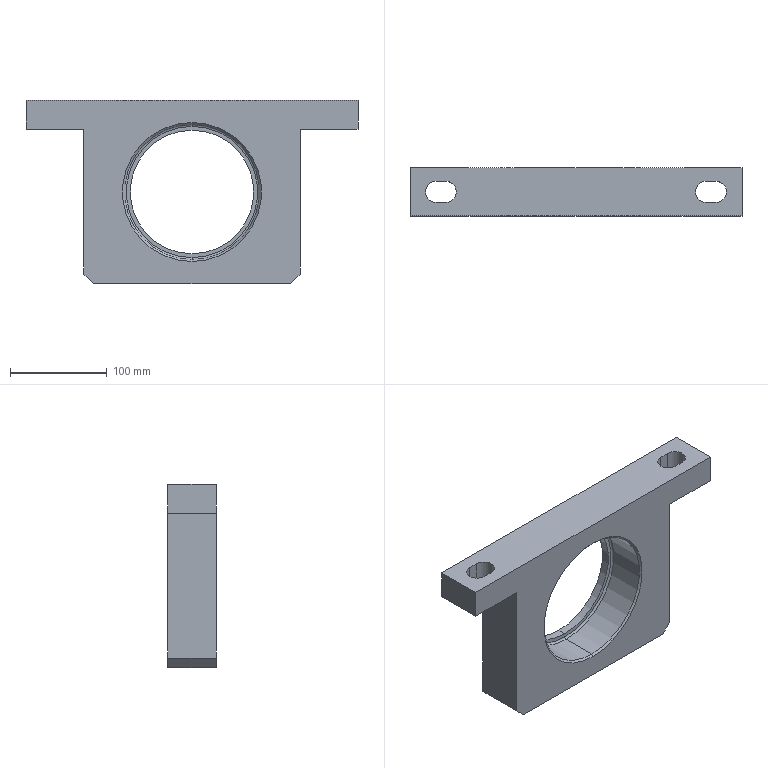Part | SolidWorks | features ICE 3, Chamfer 2, Extrusion 1, Fillet 1 | 1 solid | 31 faces | box 344 x 50 x 190 mm | volume 1518259 mm3 | plane 17 | cylinder 10 | torus 2 | cone 2 | commonest cylinder face diameters 22 x6 128 x2 140 x2
STEP:
#1=CARTESIAN_POINT('',(-156.,0.,0.));
#2=VERTEX_POINT('',#1);
#3=CARTESIAN_POINT('',(-145.,11.,0.));
#4=VERTEX_POINT('',#3);
#5=CARTESIAN_POINT('',(-145.,0.,0.));
#6=DIRECTION('',(0.,0.,-1.));
#7=DIRECTION('',(-1.,0.,0.));
#8=AXIS2_PLACEMENT_3D('',#5,#6,#7);
#9=CIRCLE('',#8,11.);
#10=EDGE_CURVE('',#2,#4,#9,.T.);
#11=ORIENTED_EDGE('',*,*,#10,.F.);
#12=CARTESIAN_POINT('',(-156.,0.,-30.));
#13=VERTEX_POINT('',#12);
#14=CARTESIAN_POINT('',(-156.,0.,11.5));
#15=DIRECTION('',(0.,0.,-1.));
#16=VECTOR('',#15,1000.);
#17=LINE('',#14,#16);
#18=EDGE_CURVE('',#2,#13,#17,.T.);
#19=ORIENTED_EDGE('',*,*,#18,.T.);
#20=CARTESIAN_POINT('',(-145.,11.,-30.));
#21=VERTEX_POINT('',#20);
#22=CARTESIAN_POINT('',(-145.,0.,-30.));
#23=DIRECTION('',(0.,0.,-1.));
#24=DIRECTION('',(-1.,0.,0.));
#25=AXIS2_PLACEMENT_3D('',#22,#23,#24);
#26=CIRCLE('',#25,11.);
#27=EDGE_CURVE('',#13,#21,#26,.T.);
#28=ORIENTED_EDGE('',*,*,#27,.T.);
#29=CARTESIAN_POINT('',(-145.,11.,11.5));
#30=DIRECTION('',(0.,0.,-1.));
#31=VECTOR('',#30,1000.);
#32=LINE('',#29,#31);
#33=EDGE_CURVE('',#4,#21,#32,.T.);
#34=ORIENTED_EDGE('',*,*,#33,.F.);
#35=EDGE_LOOP('',(#11,#19,#28,#34));
#36=FACE_OUTER_BOUND('',#35,.T.);
#37=CARTESIAN_POINT('',(-145.,0.,11.5));
#38=DIRECTION('',(0.,0.,-1.));
#39=DIRECTION('',(-1.,0.,0.));
#40=AXIS2_PLACEMENT_3D('',#37,#38,#39);
#41=CYLINDRICAL_SURFACE('',#40,11.);
#42=ADVANCED_FACE('',(#36),#41,.F.);
#43=CARTESIAN_POINT('',(124.,0.,0.));
#44=VERTEX_POINT('',#43);
#45=CARTESIAN_POINT('',(135.,11.,0.));
#46=VERTEX_POINT('',#45);
#47=CARTESIAN_POINT('',(135.,0.,0.));
#48=DIRECTION('',(0.,0.,-1.));
#49=DIRECTION('',(-1.,0.,0.));
#50=AXIS2_PLACEMENT_3D('',#47,#48,#49);
#51=CIRCLE('',#50,11.);
#52=EDGE_CURVE('',#44,#46,#51,.T.);
#53=ORIENTED_EDGE('',*,*,#52,.F.);
#54=CARTESIAN_POINT('',(124.,0.,-30.));
#55=VERTEX_POINT('',#54);
#56=CARTESIAN_POINT('',(124.,0.,11.5));
#57=DIRECTION('',(0.,0.,-1.));
#58=VECTOR('',#57,1000.);
#59=LINE('',#56,#58);
#60=EDGE_CURVE('',#44,#55,#59,.T.);
#61=ORIENTED_EDGE('',*,*,#60,.T.);
#62=CARTESIAN_POINT('',(135.,11.,-30.));
#63=VERTEX_POINT('',#62);
#64=CARTESIAN_POINT('',(135.,0.,-30.));
#65=DIRECTION('',(0.,0.,-1.));
#66=DIRECTION('',(-1.,0.,0.));
#67=AXIS2_PLACEMENT_3D('',#64,#65,#66);
#68=CIRCLE('',#67,11.);
#69=EDGE_CURVE('',#55,#63,#68,.T.);
#70=ORIENTED_EDGE('',*,*,#69,.T.);
#71=CARTESIAN_POINT('',(135.,11.,11.5));
#72=DIRECTION('',(0.,0.,-1.));
#73=VECTOR('',#72,1000.);
#74=LINE('',#71,#73);
#75=EDGE_CURVE('',#46,#63,#74,.T.);
#76=ORIENTED_EDGE('',*,*,#75,.F.);
#77=EDGE_LOOP('',(#53,#61,#70,#76));
#78=FACE_OUTER_BOUND('',#77,.T.);
#79=CARTESIAN_POINT('',(135.,0.,11.5));
#80=DIRECTION('',(0.,0.,-1.));
#81=DIRECTION('',(-1.,0.,0.));
#82=AXIS2_PLACEMENT_3D('',#79,#80,#81);
#83=CYLINDRICAL_SURFACE('',#82,11.);
#84=ADVANCED_FACE('',(#78),#83,.F.);
#85=CARTESIAN_POINT('',(0.,16.5,-27.));
#86=VERTEX_POINT('',#85);
#87=CARTESIAN_POINT('',(0.,16.5,-163.));
#88=VERTEX_POINT('',#87);
#89=CARTESIAN_POINT('',(0.,16.5,-95.));
#90=DIRECTION('',(0.,-1.,0.));
#91=DIRECTION('',(0.,0.,-1.));
#92=AXIS2_PLACEMENT_3D('',#89,#90,#91);
#93=CIRCLE('',#92,68.);
#94=EDGE_CURVE('',#86,#88,#93,.T.);
#95=ORIENTED_EDGE('',*,*,#94,.F.);
#96=CARTESIAN_POINT('',(0.,14.5,-25.));
#97=VERTEX_POINT('',#96);
#98=CARTESIAN_POINT('',(0.,14.5,-27.));
#99=DIRECTION('',(1.,0.,0.));
#100=DIRECTION('',(0.,0.,-1.));
#101=AXIS2_PLACEMENT_3D('',#98,#99,#100);
#102=CIRCLE('',#101,2.);
#103=EDGE_CURVE('',#86,#97,#102,.T.);
#104=ORIENTED_EDGE('',*,*,#103,.T.);
#105=CARTESIAN_POINT('',(0.,14.5,-165.));
#106=VERTEX_POINT('',#105);
#107=CARTESIAN_POINT('',(0.,14.5,-95.));
#108=DIRECTION('',(0.,1.,0.));
#109=DIRECTION('',(0.,0.,-1.));
#110=AXIS2_PLACEMENT_3D('',#107,#108,#109);
#111=CIRCLE('',#110,70.);
#112=EDGE_CURVE('',#106,#97,#111,.T.);
#113=ORIENTED_EDGE('',*,*,#112,.F.);
#114=CARTESIAN_POINT('',(0.,14.5,-163.));
#115=DIRECTION('',(-1.,0.,0.));
#116=DIRECTION('',(0.,0.,1.));
#117=AXIS2_PLACEMENT_3D('',#114,#115,#116);
#118=CIRCLE('',#117,2.);
#119=EDGE_CURVE('',#88,#106,#118,.T.);
#120=ORIENTED_EDGE('',*,*,#119,.F.);
#121=EDGE_LOOP('',(#95,#104,#113,#120));
#122=FACE_OUTER_BOUND('',#121,.T.);
#123=CARTESIAN_POINT('',(0.,14.5,-95.));
#124=DIRECTION('',(0.,-1.,0.));
#125=DIRECTION('',(0.,0.,-1.));
#126=AXIS2_PLACEMENT_3D('',#123,#124,#125);
#127=TOROIDAL_SURFACE('',#126,68.,2.);
#128=ADVANCED_FACE('',(#122),#127,.F.);
#129=CARTESIAN_POINT('',(0.,-23.,-25.));
#130=VERTEX_POINT('',#129);
#131=CARTESIAN_POINT('',(0.,-23.,-165.));
#132=VERTEX_POINT('',#131);
#133=CARTESIAN_POINT('',(0.,-23.,-95.));
#134=DIRECTION('',(0.,-1.,0.));
#135=DIRECTION('',(0.,0.,1.));
#136=AXIS2_PLACEMENT_3D('',#133,#134,#135);
#137=CIRCLE('',#136,70.);
#138=EDGE_CURVE('',#130,#132,#137,.T.);
#139=ORIENTED_EDGE('',*,*,#138,.F.);
#140=CARTESIAN_POINT('',(0.,-25.,-23.));
#141=VERTEX_POINT('',#140);
#142=CARTESIAN_POINT('',(0.,-23.,-25.));
#143=DIRECTION('',(0.,-0.7071,0.7071));
#144=VECTOR('',#143,1000.);
#145=LINE('',#142,#144);
#146=EDGE_CURVE('',#130,#141,#145,.T.);
#147=ORIENTED_EDGE('',*,*,#146,.T.);
#148=CARTESIAN_POINT('',(0.,-25.,-167.));
#149=VERTEX_POINT('',#148);
#150=CARTESIAN_POINT('',(0.,-25.,-95.));
#151=DIRECTION('',(0.,1.,0.));
#152=DIRECTION('',(0.,0.,1.));
#153=AXIS2_PLACEMENT_3D('',#150,#151,#152);
#154=CIRCLE('',#153,72.);
#155=EDGE_CURVE('',#149,#141,#154,.T.);
#156=ORIENTED_EDGE('',*,*,#155,.F.);
#157=CARTESIAN_POINT('',(0.,-23.,-165.));
#158=DIRECTION('',(0.,-0.7071,-0.7071));
#159=VECTOR('',#158,1000.);
#160=LINE('',#157,#159);
#161=EDGE_CURVE('',#132,#149,#160,.T.);
#162=ORIENTED_EDGE('',*,*,#161,.F.);
#163=EDGE_LOOP('',(#139,#147,#156,#162));
#164=FACE_OUTER_BOUND('',#163,.T.);
#165=CARTESIAN_POINT('',(0.,-23.,-95.));
#166=DIRECTION('',(0.,-1.,0.));
#167=DIRECTION('',(0.,0.,-1.));
#168=AXIS2_PLACEMENT_3D('',#165,#166,#167);
#169=CONICAL_SURFACE('',#168,70.,0.7854);
#170=ADVANCED_FACE('',(#164),#169,.F.);
#171=ORIENTED_EDGE('',*,*,#112,.T.);
#172=CARTESIAN_POINT('',(0.,16.5,-25.));
#173=DIRECTION('',(0.,-1.,0.));
#174=VECTOR('',#173,1000.);
#175=LINE('',#172,#174);
#176=EDGE_CURVE('',#97,#130,#175,.T.);
#177=ORIENTED_EDGE('',*,*,#176,.T.);
#178=ORIENTED_EDGE('',*,*,#138,.T.);
#179=CARTESIAN_POINT('',(0.,16.5,-165.));
#180=DIRECTION('',(0.,-1.,0.));
#181=VECTOR('',#180,1000.);
#182=LINE('',#179,#181);
#183=EDGE_CURVE('',#106,#132,#182,.T.);
#184=ORIENTED_EDGE('',*,*,#183,.F.);
#185=EDGE_LOOP('',(#171,#177,#178,#184));
#186=FACE_OUTER_BOUND('',#185,.T.);
#187=CARTESIAN_POINT('',(0.,16.5,-95.));
#188=DIRECTION('',(0.,-1.,0.));
#189=DIRECTION('',(0.,0.,-1.));
#190=AXIS2_PLACEMENT_3D('',#187,#188,#189);
#191=CYLINDRICAL_SURFACE('',#190,70.);
#192=ADVANCED_FACE('',(#186),#191,.F.);
#193=CARTESIAN_POINT('',(0.,25.,-159.));
#194=VERTEX_POINT('',#193);
#195=CARTESIAN_POINT('',(0.,25.,-31.));
#196=VERTEX_POINT('',#195);
#197=CARTESIAN_POINT('',(0.,25.,-95.));
#198=DIRECTION('',(0.,1.,0.));
#199=DIRECTION('',(0.,0.,1.));
#200=AXIS2_PLACEMENT_3D('',#197,#198,#199);
#201=CIRCLE('',#200,64.);
#202=EDGE_CURVE('',#194,#196,#201,.T.);
#203=ORIENTED_EDGE('',*,*,#202,.T.);
#204=CARTESIAN_POINT('',(0.,16.5,-31.));
#205=VERTEX_POINT('',#204);
#206=CARTESIAN_POINT('',(0.,25.,-31.));
#207=DIRECTION('',(0.,-1.,0.));
#208=VECTOR('',#207,1000.);
#209=LINE('',#206,#208);
#210=EDGE_CURVE('',#196,#205,#209,.T.);
#211=ORIENTED_EDGE('',*,*,#210,.T.);
#212=CARTESIAN_POINT('',(0.,16.5,-159.));
#213=VERTEX_POINT('',#212);
#214=CARTESIAN_POINT('',(0.,16.5,-95.));
#215=DIRECTION('',(0.,-1.,0.));
#216=DIRECTION('',(0.,0.,-1.));
#217=AXIS2_PLACEMENT_3D('',#214,#215,#216);
#218=CIRCLE('',#217,64.);
#219=EDGE_CURVE('',#205,#213,#218,.T.);
#220=ORIENTED_EDGE('',*,*,#219,.T.);
#221=CARTESIAN_POINT('',(0.,25.,-159.));
#222=DIRECTION('',(0.,-1.,0.));
#223=VECTOR('',#222,1000.);
#224=LINE('',#221,#223);
#225=EDGE_CURVE('',#194,#213,#224,.T.);
#226=ORIENTED_EDGE('',*,*,#225,.F.);
#227=EDGE_LOOP('',(#203,#211,#220,#226));
#228=FACE_OUTER_BOUND('',#227,.T.);
#229=CARTESIAN_POINT('',(0.,25.,-95.));
#230=DIRECTION('',(0.,-1.,0.));
#231=DIRECTION('',(0.,0.,-1.));
#232=AXIS2_PLACEMENT_3D('',#229,#230,#231);
#233=CYLINDRICAL_SURFACE('',#232,64.);
#234=ADVANCED_FACE('',(#228),#233,.F.);
#235=ORIENTED_EDGE('',*,*,#210,.F.);
#236=CARTESIAN_POINT('',(0.,25.,-95.));
#237=DIRECTION('',(0.,1.,0.));
#238=DIRECTION('',(0.,0.,1.));
#239=AXIS2_PLACEMENT_3D('',#236,#237,#238);
#240=CIRCLE('',#239,64.);
#241=EDGE_CURVE('',#196,#194,#240,.T.);
#242=ORIENTED_EDGE('',*,*,#241,.T.);
#243=ORIENTED_EDGE('',*,*,#225,.T.);
#244=CARTESIAN_POINT('',(0.,16.5,-95.));
#245=DIRECTION('',(0.,-1.,0.));
#246=DIRECTION('',(0.,0.,-1.));
#247=AXIS2_PLACEMENT_3D('',#244,#245,#246);
#248=CIRCLE('',#247,64.);
#249=EDGE_CURVE('',#213,#205,#248,.T.);
#250=ORIENTED_EDGE('',*,*,#249,.T.);
#251=EDGE_LOOP('',(#235,#242,#243,#250));
#252=FACE_OUTER_BOUND('',#251,.T.);
#253=CARTESIAN_POINT('',(0.,25.,-95.));
#254=DIRECTION('',(0.,-1.,0.));
#255=DIRECTION('',(0.,0.,-1.));
#256=AXIS2_PLACEMENT_3D('',#253,#254,#255);
#257=CYLINDRICAL_SURFACE('',#256,64.);
#258=ADVANCED_FACE('',(#252),#257,.F.);
#259=CARTESIAN_POINT('',(-102.,25.,-190.));
#260=VERTEX_POINT('',#259);
#261=CARTESIAN_POINT('',(102.,25.,-190.));
#262=VERTEX_POINT('',#261);
#263=CARTESIAN_POINT('',(-112.,25.,-190.));
#264=DIRECTION('',(1.,0.,0.));
#265=VECTOR('',#264,1000.);
#266=LINE('',#263,#265);
#267=EDGE_CURVE('',#260,#262,#266,.T.);
#268=ORIENTED_EDGE('',*,*,#267,.F.);
#269=CARTESIAN_POINT('',(-112.,25.,-180.));
#270=VERTEX_POINT('',#269);
#271=CARTESIAN_POINT('',(-98.5,25.,-193.5));
#272=DIRECTION('',(-0.7071,0.,0.7071));
#273=VECTOR('',#272,1000.);
#274=LINE('',#271,#273);
#275=EDGE_CURVE('',#260,#270,#274,.T.);
#276=ORIENTED_EDGE('',*,*,#275,.T.);
#277=CARTESIAN_POINT('',(-112.,25.,-30.));
#278=VERTEX_POINT('',#277);
#279=CARTESIAN_POINT('',(-112.,25.,-30.));
#280=DIRECTION('',(0.,0.,-1.));
#281=VECTOR('',#280,1000.);
#282=LINE('',#279,#281);
#283=EDGE_CURVE('',#278,#270,#282,.T.);
#284=ORIENTED_EDGE('',*,*,#283,.F.);
#285=CARTESIAN_POINT('',(-172.,25.,-30.));
#286=VERTEX_POINT('',#285);
#287=CARTESIAN_POINT('',(-172.,25.,-30.));
#288=DIRECTION('',(-1.,0.,0.));
#289=VECTOR('',#288,1000.);
#290=LINE('',#287,#289);
#291=EDGE_CURVE('',#278,#286,#290,.T.);
#292=ORIENTED_EDGE('',*,*,#291,.T.);
#293=CARTESIAN_POINT('',(-172.,25.,0.));
#294=VERTEX_POINT('',#293);
#295=CARTESIAN_POINT('',(-172.,25.,0.));
#296=DIRECTION('',(0.,0.,1.));
#297=VECTOR('',#296,1000.);
#298=LINE('',#295,#297);
#299=EDGE_CURVE('',#286,#294,#298,.T.);
#300=ORIENTED_EDGE('',*,*,#299,.T.);
#301=CARTESIAN_POINT('',(172.,25.,0.));
#302=VERTEX_POINT('',#301);
#303=CARTESIAN_POINT('',(-172.,25.,0.));
#304=DIRECTION('',(1.,0.,0.));
#305=VECTOR('',#304,1000.);
#306=LINE('',#303,#305);
#307=EDGE_CURVE('',#294,#302,#306,.T.);
#308=ORIENTED_EDGE('',*,*,#307,.T.);
#309=CARTESIAN_POINT('',(172.,25.,-30.));
#310=VERTEX_POINT('',#309);
#311=CARTESIAN_POINT('',(172.,25.,0.));
#312=DIRECTION('',(0.,0.,-1.));
#313=VECTOR('',#312,1000.);
#314=LINE('',#311,#313);
#315=EDGE_CURVE('',#302,#310,#314,.T.);
#316=ORIENTED_EDGE('',*,*,#315,.T.);
#317=CARTESIAN_POINT('',(112.,25.,-30.));
#318=VERTEX_POINT('',#317);
#319=CARTESIAN_POINT('',(172.,25.,-30.));
#320=DIRECTION('',(-1.,0.,0.));
#321=VECTOR('',#320,1000.);
#322=LINE('',#319,#321);
#323=EDGE_CURVE('',#310,#318,#322,.T.);
#324=ORIENTED_EDGE('',*,*,#323,.T.);
#325=CARTESIAN_POINT('',(112.,25.,-180.));
#326=VERTEX_POINT('',#325);
#327=CARTESIAN_POINT('',(112.,25.,-30.));
#328=DIRECTION('',(0.,0.,1.));
#329=VECTOR('',#328,1000.);
#330=LINE('',#327,#329);
#331=EDGE_CURVE('',#326,#318,#330,.T.);
#332=ORIENTED_EDGE('',*,*,#331,.F.);
#333=CARTESIAN_POINT('',(98.5,25.,-193.5));
#334=DIRECTION('',(-0.7071,0.,-0.7071));
#335=VECTOR('',#334,1000.);
#336=LINE('',#333,#335);
#337=EDGE_CURVE('',#326,#262,#336,.T.);
#338=ORIENTED_EDGE('',*,*,#337,.T.);
#339=EDGE_LOOP('',(#268,#276,#284,#292,#300,#308,#316,#324,#332,#338));
#340=FACE_OUTER_BOUND('',#339,.T.);
#341=ORIENTED_EDGE('',*,*,#202,.F.);
#342=ORIENTED_EDGE('',*,*,#241,.F.);
#343=EDGE_LOOP('',(#341,#342));
#344=FACE_BOUND('',#343,.T.);
#345=CARTESIAN_POINT('',(0.,25.,-95.));
#346=DIRECTION('',(0.,1.,0.));
#347=DIRECTION('',(0.,0.,1.));
#348=AXIS2_PLACEMENT_3D('',#345,#346,#347);
#349=PLANE('',#348);
#350=ADVANCED_FACE('',(#340,#344),#349,.T.);
#351=ORIENTED_EDGE('',*,*,#155,.T.);
#352=CARTESIAN_POINT('',(0.,-25.,-95.));
#353=DIRECTION('',(0.,1.,0.));
#354=DIRECTION('',(0.,0.,1.));
#355=AXIS2_PLACEMENT_3D('',#352,#353,#354);
#356=CIRCLE('',#355,72.);
#357=EDGE_CURVE('',#141,#149,#356,.T.);
#358=ORIENTED_EDGE('',*,*,#357,.T.);
#359=EDGE_LOOP('',(#351,#358));
#360=FACE_BOUND('',#359,.T.);
#361=CARTESIAN_POINT('',(-112.,-25.,-30.));
#362=VERTEX_POINT('',#361);
#363=CARTESIAN_POINT('',(-112.,-25.,-180.));
#364=VERTEX_POINT('',#363);
#365=CARTESIAN_POINT('',(-112.,-25.,-30.));
#366=DIRECTION('',(0.,0.,-1.));
#367=VECTOR('',#366,1000.);
#368=LINE('',#365,#367);
#369=EDGE_CURVE('',#362,#364,#368,.T.);
#370=ORIENTED_EDGE('',*,*,#369,.T.);
#371=CARTESIAN_POINT('',(-102.,-25.,-190.));
#372=VERTEX_POINT('',#371);
#373=CARTESIAN_POINT('',(-112.,-25.,-180.));
#374=DIRECTION('',(0.7071,0.,-0.7071));
#375=VECTOR('',#374,1000.);
#376=LINE('',#373,#375);
#377=EDGE_CURVE('',#364,#372,#376,.T.);
#378=ORIENTED_EDGE('',*,*,#377,.T.);
#379=CARTESIAN_POINT('',(102.,-25.,-190.));
#380=VERTEX_POINT('',#379);
#381=CARTESIAN_POINT('',(-112.,-25.,-190.));
#382=DIRECTION('',(1.,0.,0.));
#383=VECTOR('',#382,1000.);
#384=LINE('',#381,#383);
#385=EDGE_CURVE('',#372,#380,#384,.T.);
#386=ORIENTED_EDGE('',*,*,#385,.T.);
#387=CARTESIAN_POINT('',(112.,-25.,-180.));
#388=VERTEX_POINT('',#387);
#389=CARTESIAN_POINT('',(102.,-25.,-190.));
#390=DIRECTION('',(0.7071,0.,0.7071));
#391=VECTOR('',#390,1000.);
#392=LINE('',#389,#391);
#393=EDGE_CURVE('',#380,#388,#392,.T.);
#394=ORIENTED_EDGE('',*,*,#393,.T.);
#395=CARTESIAN_POINT('',(112.,-25.,-30.));
#396=VERTEX_POINT('',#395);
#397=CARTESIAN_POINT('',(112.,-25.,-30.));
#398=DIRECTION('',(0.,0.,1.));
#399=VECTOR('',#398,1000.);
#400=LINE('',#397,#399);
#401=EDGE_CURVE('',#388,#396,#400,.T.);
#402=ORIENTED_EDGE('',*,*,#401,.T.);
#403=CARTESIAN_POINT('',(172.,-25.,-30.));
#404=VERTEX_POINT('',#403);
#405=CARTESIAN_POINT('',(172.,-25.,-30.));
#406=DIRECTION('',(-1.,0.,0.));
#407=VECTOR('',#406,1000.);
#408=LINE('',#405,#407);
#409=EDGE_CURVE('',#404,#396,#408,.T.);
#410=ORIENTED_EDGE('',*,*,#409,.F.);
#411=CARTESIAN_POINT('',(172.,-25.,0.));
#412=VERTEX_POINT('',#411);
#413=CARTESIAN_POINT('',(172.,-25.,0.));
#414=DIRECTION('',(0.,0.,-1.));
#415=VECTOR('',#414,1000.);
#416=LINE('',#413,#415);
#417=EDGE_CURVE('',#412,#404,#416,.T.);
#418=ORIENTED_EDGE('',*,*,#417,.F.);
#419=CARTESIAN_POINT('',(-172.,-25.,0.));
#420=VERTEX_POINT('',#419);
#421=CARTESIAN_POINT('',(-172.,-25.,0.));
#422=DIRECTION('',(1.,0.,0.));
#423=VECTOR('',#422,1000.);
#424=LINE('',#421,#423);
#425=EDGE_CURVE('',#420,#412,#424,.T.);
#426=ORIENTED_EDGE('',*,*,#425,.F.);
#427=CARTESIAN_POINT('',(-172.,-25.,-30.));
#428=VERTEX_POINT('',#427);
#429=CARTESIAN_POINT('',(-172.,-25.,0.));
#430=DIRECTION('',(0.,0.,1.));
#431=VECTOR('',#430,1000.);
#432=LINE('',#429,#431);
#433=EDGE_CURVE('',#428,#420,#432,.T.);
#434=ORIENTED_EDGE('',*,*,#433,.F.);
#435=CARTESIAN_POINT('',(-172.,-25.,-30.));
#436=DIRECTION('',(-1.,0.,0.));
#437=VECTOR('',#436,1000.);
#438=LINE('',#435,#437);
#439=EDGE_CURVE('',#362,#428,#438,.T.);
#440=ORIENTED_EDGE('',*,*,#439,.F.);
#441=EDGE_LOOP('',(#370,#378,#386,#394,#402,#410,#418,#426,#434,#440));
#442=FACE_OUTER_BOUND('',#441,.T.);
#443=CARTESIAN_POINT('',(0.,-25.,-95.));
#444=DIRECTION('',(0.,1.,0.));
#445=DIRECTION('',(0.,0.,1.));
#446=AXIS2_PLACEMENT_3D('',#443,#444,#445);
#447=PLANE('',#446);
#448=ADVANCED_FACE('',(#360,#442),#447,.F.);
#449=ORIENTED_EDGE('',*,*,#417,.T.);
#450=CARTESIAN_POINT('',(172.,25.,-30.));
#451=DIRECTION('',(0.,-1.,0.));
#452=VECTOR('',#451,1000.);
#453=LINE('',#450,#452);
#454=EDGE_CURVE('',#310,#404,#453,.T.);
#455=ORIENTED_EDGE('',*,*,#454,.F.);
#456=ORIENTED_EDGE('',*,*,#315,.F.);
#457=CARTESIAN_POINT('',(172.,25.,0.));
#458=DIRECTION('',(0.,-1.,0.));
#459=VECTOR('',#458,1000.);
#460=LINE('',#457,#459);
#461=EDGE_CURVE('',#302,#412,#460,.T.);
#462=ORIENTED_EDGE('',*,*,#461,.T.);
#463=EDGE_LOOP('',(#449,#455,#456,#462));
#464=FACE_OUTER_BOUND('',#463,.T.);
#465=CARTESIAN_POINT('',(172.,25.,0.));
#466=DIRECTION('',(-1.,0.,0.));
#467=DIRECTION('',(0.,0.,1.));
#468=AXIS2_PLACEMENT_3D('',#465,#466,#467);
#469=PLANE('',#468);
#470=ADVANCED_FACE('',(#464),#469,.F.);
#471=CARTESIAN_POINT('',(145.,-11.,-30.));
#472=VERTEX_POINT('',#471);
#473=CARTESIAN_POINT('',(135.,-11.,-30.));
#474=VERTEX_POINT('',#473);
#475=CARTESIAN_POINT('',(145.,-11.,-30.));
#476=DIRECTION('',(-1.,0.,0.));
#477=VECTOR('',#476,1000.);
#478=LINE('',#475,#477);
#479=EDGE_CURVE('',#472,#474,#478,.T.);
#480=ORIENTED_EDGE('',*,*,#479,.F.);
#481=CARTESIAN_POINT('',(145.,11.,-30.));
#482=VERTEX_POINT('',#481);
#483=CARTESIAN_POINT('',(145.,0.,-30.));
#484=DIRECTION('',(0.,0.,-1.));
#485=DIRECTION('',(-1.,0.,0.));
#486=AXIS2_PLACEMENT_3D('',#483,#484,#485);
#487=CIRCLE('',#486,11.);
#488=EDGE_CURVE('',#482,#472,#487,.T.);
#489=ORIENTED_EDGE('',*,*,#488,.F.);
#490=CARTESIAN_POINT('',(145.,11.,-30.));
#491=DIRECTION('',(1.,0.,0.));
#492=VECTOR('',#491,1000.);
#493=LINE('',#490,#492);
#494=EDGE_CURVE('',#63,#482,#493,.T.);
#495=ORIENTED_EDGE('',*,*,#494,.F.);
#496=ORIENTED_EDGE('',*,*,#69,.F.);
#497=CARTESIAN_POINT('',(135.,0.,-30.));
#498=DIRECTION('',(0.,0.,-1.));
#499=DIRECTION('',(-1.,0.,0.));
#500=AXIS2_PLACEMENT_3D('',#497,#498,#499);
#501=CIRCLE('',#500,11.);
#502=EDGE_CURVE('',#474,#55,#501,.T.);
#503=ORIENTED_EDGE('',*,*,#502,.F.);
#504=EDGE_LOOP('',(#480,#489,#495,#496,#503));
#505=FACE_BOUND('',#504,.T.);
#506=ORIENTED_EDGE('',*,*,#409,.T.);
#507=CARTESIAN_POINT('',(112.,25.,-30.));
#508=DIRECTION('',(0.,-1.,0.));
#509=VECTOR('',#508,1000.);
#510=LINE('',#507,#509);
#511=EDGE_CURVE('',#318,#396,#510,.T.);
#512=ORIENTED_EDGE('',*,*,#511,.F.);
#513=ORIENTED_EDGE('',*,*,#323,.F.);
#514=ORIENTED_EDGE('',*,*,#454,.T.);
#515=EDGE_LOOP('',(#506,#512,#513,#514));
#516=FACE_OUTER_BOUND('',#515,.T.);
#517=CARTESIAN_POINT('',(172.,25.,-30.));
#518=DIRECTION('',(0.,0.,1.));
#519=DIRECTION('',(1.,0.,0.));
#520=AXIS2_PLACEMENT_3D('',#517,#518,#519);
#521=PLANE('',#520);
#522=ADVANCED_FACE('',(#505,#516),#521,.F.);
#523=CARTESIAN_POINT('',(-135.,-11.,-30.));
#524=VERTEX_POINT('',#523);
#525=CARTESIAN_POINT('',(-145.,-11.,-30.));
#526=VERTEX_POINT('',#525);
#527=CARTESIAN_POINT('',(-135.,-11.,-30.));
#528=DIRECTION('',(-1.,0.,0.));
#529=VECTOR('',#528,1000.);
#530=LINE('',#527,#529);
#531=EDGE_CURVE('',#524,#526,#530,.T.);
#532=ORIENTED_EDGE('',*,*,#531,.F.);
#533=CARTESIAN_POINT('',(-135.,11.,-30.));
#534=VERTEX_POINT('',#533);
#535=CARTESIAN_POINT('',(-135.,0.,-30.));
#536=DIRECTION('',(0.,0.,-1.));
#537=DIRECTION('',(-1.,0.,0.));
#538=AXIS2_PLACEMENT_3D('',#535,#536,#537);
#539=CIRCLE('',#538,11.);
#540=EDGE_CURVE('',#534,#524,#539,.T.);
#541=ORIENTED_EDGE('',*,*,#540,.F.);
#542=CARTESIAN_POINT('',(-135.,11.,-30.));
#543=DIRECTION('',(1.,0.,0.));
#544=VECTOR('',#543,1000.);
#545=LINE('',#542,#544);
#546=EDGE_CURVE('',#21,#534,#545,.T.);
#547=ORIENTED_EDGE('',*,*,#546,.F.);
#548=ORIENTED_EDGE('',*,*,#27,.F.);
#549=CARTESIAN_POINT('',(-145.,0.,-30.));
#550=DIRECTION('',(0.,0.,-1.));
#551=DIRECTION('',(-1.,0.,0.));
#552=AXIS2_PLACEMENT_3D('',#549,#550,#551);
#553=CIRCLE('',#552,11.);
#554=EDGE_CURVE('',#526,#13,#553,.T.);
#555=ORIENTED_EDGE('',*,*,#554,.F.);
#556=EDGE_LOOP('',(#532,#541,#547,#548,#555));
#557=FACE_BOUND('',#556,.T.);
#558=ORIENTED_EDGE('',*,*,#439,.T.);
#559=CARTESIAN_POINT('',(-172.,25.,-30.));
#560=DIRECTION('',(0.,-1.,0.));
#561=VECTOR('',#560,1000.);
#562=LINE('',#559,#561);
#563=EDGE_CURVE('',#286,#428,#562,.T.);
#564=ORIENTED_EDGE('',*,*,#563,.F.);
#565=ORIENTED_EDGE('',*,*,#291,.F.);
#566=CARTESIAN_POINT('',(-112.,25.,-30.));
#567=DIRECTION('',(0.,-1.,0.));
#568=VECTOR('',#567,1000.);
#569=LINE('',#566,#568);
#570=EDGE_CURVE('',#278,#362,#569,.T.);
#571=ORIENTED_EDGE('',*,*,#570,.T.);
#572=EDGE_LOOP('',(#558,#564,#565,#571));
#573=FACE_OUTER_BOUND('',#572,.T.);
#574=CARTESIAN_POINT('',(-172.,25.,-30.));
#575=DIRECTION('',(0.,0.,1.));
#576=DIRECTION('',(1.,0.,0.));
#577=AXIS2_PLACEMENT_3D('',#574,#575,#576);
#578=PLANE('',#577);
#579=ADVANCED_FACE('',(#557,#573),#578,.F.);
#580=ORIENTED_EDGE('',*,*,#433,.T.);
#581=CARTESIAN_POINT('',(-172.,25.,0.));
#582=DIRECTION('',(0.,-1.,0.));
#583=VECTOR('',#582,1000.);
#584=LINE('',#581,#583);
#585=EDGE_CURVE('',#294,#420,#584,.T.);
#586=ORIENTED_EDGE('',*,*,#585,.F.);
#587=ORIENTED_EDGE('',*,*,#299,.F.);
#588=ORIENTED_EDGE('',*,*,#563,.T.);
#589=EDGE_LOOP('',(#580,#586,#587,#588));
#590=FACE_OUTER_BOUND('',#589,.T.);
#591=CARTESIAN_POINT('',(-172.,25.,0.));
#592=DIRECTION('',(1.,0.,0.));
#593=DIRECTION('',(0.,0.,-1.));
#594=AXIS2_PLACEMENT_3D('',#591,#592,#593);
#595=PLANE('',#594);
#596=ADVANCED_FACE('',(#590),#595,.F.);
#597=CARTESIAN_POINT('',(-135.,11.,0.));
#598=VERTEX_POINT('',#597);
#599=CARTESIAN_POINT('',(-172.,11.,0.));
#600=DIRECTION('',(1.,0.,0.));
#601=VECTOR('',#600,1000.);
#602=LINE('',#599,#601);
#603=EDGE_CURVE('',#4,#598,#602,.T.);
#604=ORIENTED_EDGE('',*,*,#603,.T.);
#605=CARTESIAN_POINT('',(-135.,-11.,0.));
#606=VERTEX_POINT('',#605);
#607=CARTESIAN_POINT('',(-135.,0.,0.));
#608=DIRECTION('',(0.,0.,-1.));
#609=DIRECTION('',(-1.,0.,0.));
#610=AXIS2_PLACEMENT_3D('',#607,#608,#609);
#611=CIRCLE('',#610,11.);
#612=EDGE_CURVE('',#598,#606,#611,.T.);
#613=ORIENTED_EDGE('',*,*,#612,.T.);
#614=CARTESIAN_POINT('',(-145.,-11.,0.));
#615=VERTEX_POINT('',#614);
#616=CARTESIAN_POINT('',(-172.,-11.,0.));
#617=DIRECTION('',(-1.,0.,0.));
#618=VECTOR('',#617,1000.);
#619=LINE('',#616,#618);
#620=EDGE_CURVE('',#606,#615,#619,.T.);
#621=ORIENTED_EDGE('',*,*,#620,.T.);
#622=CARTESIAN_POINT('',(-145.,0.,0.));
#623=DIRECTION('',(0.,0.,-1.));
#624=DIRECTION('',(-1.,0.,0.));
#625=AXIS2_PLACEMENT_3D('',#622,#623,#624);
#626=CIRCLE('',#625,11.);
#627=EDGE_CURVE('',#615,#2,#626,.T.);
#628=ORIENTED_EDGE('',*,*,#627,.T.);
#629=ORIENTED_EDGE('',*,*,#10,.T.);
#630=EDGE_LOOP('',(#604,#613,#621,#628,#629));
#631=FACE_BOUND('',#630,.T.);
#632=CARTESIAN_POINT('',(145.,11.,0.));
#633=VERTEX_POINT('',#632);
#634=CARTESIAN_POINT('',(-172.,11.,0.));
#635=DIRECTION('',(1.,0.,0.));
#636=VECTOR('',#635,1000.);
#637=LINE('',#634,#636);
#638=EDGE_CURVE('',#46,#633,#637,.T.);
#639=ORIENTED_EDGE('',*,*,#638,.T.);
#640=CARTESIAN_POINT('',(145.,-11.,0.));
#641=VERTEX_POINT('',#640);
#642=CARTESIAN_POINT('',(145.,0.,0.));
#643=DIRECTION('',(0.,0.,-1.));
#644=DIRECTION('',(-1.,0.,0.));
#645=AXIS2_PLACEMENT_3D('',#642,#643,#644);
#646=CIRCLE('',#645,11.);
#647=EDGE_CURVE('',#633,#641,#646,.T.);
#648=ORIENTED_EDGE('',*,*,#647,.T.);
#649=CARTESIAN_POINT('',(135.,-11.,0.));
#650=VERTEX_POINT('',#649);
#651=CARTESIAN_POINT('',(-172.,-11.,0.));
#652=DIRECTION('',(-1.,0.,0.));
#653=VECTOR('',#652,1000.);
#654=LINE('',#651,#653);
#655=EDGE_CURVE('',#641,#650,#654,.T.);
#656=ORIENTED_EDGE('',*,*,#655,.T.);
#657=CARTESIAN_POINT('',(135.,0.,0.));
#658=DIRECTION('',(0.,0.,-1.));
#659=DIRECTION('',(-1.,0.,0.));
#660=AXIS2_PLACEMENT_3D('',#657,#658,#659);
#661=CIRCLE('',#660,11.);
#662=EDGE_CURVE('',#650,#44,#661,.T.);
#663=ORIENTED_EDGE('',*,*,#662,.T.);
#664=ORIENTED_EDGE('',*,*,#52,.T.);
#665=EDGE_LOOP('',(#639,#648,#656,#663,#664));
#666=FACE_BOUND('',#665,.T.);
#667=ORIENTED_EDGE('',*,*,#425,.T.);
#668=ORIENTED_EDGE('',*,*,#461,.F.);
#669=ORIENTED_EDGE('',*,*,#307,.F.);
#670=ORIENTED_EDGE('',*,*,#585,.T.);
#671=EDGE_LOOP('',(#667,#668,#669,#670));
#672=FACE_OUTER_BOUND('',#671,.T.);
#673=CARTESIAN_POINT('',(-172.,25.,0.));
#674=DIRECTION('',(0.,0.,-1.));
#675=DIRECTION('',(-1.,0.,0.));
#676=AXIS2_PLACEMENT_3D('',#673,#674,#675);
#677=PLANE('',#676);
#678=ADVANCED_FACE('',(#631,#666,#672),#677,.F.);
#679=ORIENTED_EDGE('',*,*,#176,.F.);
#680=CARTESIAN_POINT('',(0.,14.5,-95.));
#681=DIRECTION('',(0.,1.,0.));
#682=DIRECTION('',(0.,0.,-1.));
#683=AXIS2_PLACEMENT_3D('',#680,#681,#682);
#684=CIRCLE('',#683,70.);
#685=EDGE_CURVE('',#97,#106,#684,.T.);
#686=ORIENTED_EDGE('',*,*,#685,.T.);
#687=ORIENTED_EDGE('',*,*,#183,.T.);
#688=CARTESIAN_POINT('',(0.,-23.,-95.));
#689=DIRECTION('',(0.,-1.,0.));
#690=DIRECTION('',(0.,0.,1.));
#691=AXIS2_PLACEMENT_3D('',#688,#689,#690);
#692=CIRCLE('',#691,70.);
#693=EDGE_CURVE('',#132,#130,#692,.T.);
#694=ORIENTED_EDGE('',*,*,#693,.T.);
#695=EDGE_LOOP('',(#679,#686,#687,#694));
#696=FACE_OUTER_BOUND('',#695,.T.);
#697=CARTESIAN_POINT('',(0.,16.5,-95.));
#698=DIRECTION('',(0.,-1.,0.));
#699=DIRECTION('',(0.,0.,-1.));
#700=AXIS2_PLACEMENT_3D('',#697,#698,#699);
#701=CYLINDRICAL_SURFACE('',#700,70.);
#702=ADVANCED_FACE('',(#696),#701,.F.);
#703=CARTESIAN_POINT('',(0.,16.5,-95.));
#704=DIRECTION('',(0.,-1.,0.));
#705=DIRECTION('',(0.,0.,-1.));
#706=AXIS2_PLACEMENT_3D('',#703,#704,#705);
#707=CIRCLE('',#706,68.);
#708=EDGE_CURVE('',#88,#86,#707,.T.);
#709=ORIENTED_EDGE('',*,*,#708,.T.);
#710=ORIENTED_EDGE('',*,*,#94,.T.);
#711=EDGE_LOOP('',(#709,#710));
#712=FACE_OUTER_BOUND('',#711,.T.);
#713=ORIENTED_EDGE('',*,*,#249,.F.);
#714=ORIENTED_EDGE('',*,*,#219,.F.);
#715=EDGE_LOOP('',(#713,#714));
#716=FACE_BOUND('',#715,.T.);
#717=CARTESIAN_POINT('',(0.,16.5,-95.));
#718=DIRECTION('',(0.,-1.,0.));
#719=DIRECTION('',(0.,0.,-1.));
#720=AXIS2_PLACEMENT_3D('',#717,#718,#719);
#721=PLANE('',#720);
#722=ADVANCED_FACE('',(#712,#716),#721,.T.);
#723=ORIENTED_EDGE('',*,*,#146,.F.);
#724=ORIENTED_EDGE('',*,*,#693,.F.);
#725=ORIENTED_EDGE('',*,*,#161,.T.);
#726=ORIENTED_EDGE('',*,*,#357,.F.);
#727=EDGE_LOOP('',(#723,#724,#725,#726));
#728=FACE_OUTER_BOUND('',#727,.T.);
#729=CARTESIAN_POINT('',(0.,-23.,-95.));
#730=DIRECTION('',(0.,-1.,0.));
#731=DIRECTION('',(0.,0.,-1.));
#732=AXIS2_PLACEMENT_3D('',#729,#730,#731);
#733=CONICAL_SURFACE('',#732,70.,0.7854);
#734=ADVANCED_FACE('',(#728),#733,.F.);
#735=ORIENTED_EDGE('',*,*,#103,.F.);
#736=ORIENTED_EDGE('',*,*,#708,.F.);
#737=ORIENTED_EDGE('',*,*,#119,.T.);
#738=ORIENTED_EDGE('',*,*,#685,.F.);
#739=EDGE_LOOP('',(#735,#736,#737,#738));
#740=FACE_OUTER_BOUND('',#739,.T.);
#741=CARTESIAN_POINT('',(0.,14.5,-95.));
#742=DIRECTION('',(0.,-1.,0.));
#743=DIRECTION('',(0.,0.,-1.));
#744=AXIS2_PLACEMENT_3D('',#741,#742,#743);
#745=TOROIDAL_SURFACE('',#744,68.,2.);
#746=ADVANCED_FACE('',(#740),#745,.F.);
#747=CARTESIAN_POINT('',(145.,11.,11.5));
#748=DIRECTION('',(0.,0.,-1.));
#749=VECTOR('',#748,1000.);
#750=LINE('',#747,#749);
#751=EDGE_CURVE('',#633,#482,#750,.T.);
#752=ORIENTED_EDGE('',*,*,#751,.T.);
#753=ORIENTED_EDGE('',*,*,#488,.T.);
#754=CARTESIAN_POINT('',(145.,-11.,11.5));
#755=DIRECTION('',(0.,0.,-1.));
#756=VECTOR('',#755,1000.);
#757=LINE('',#754,#756);
#758=EDGE_CURVE('',#641,#472,#757,.T.);
#759=ORIENTED_EDGE('',*,*,#758,.F.);
#760=ORIENTED_EDGE('',*,*,#647,.F.);
#761=EDGE_LOOP('',(#752,#753,#759,#760));
#762=FACE_OUTER_BOUND('',#761,.T.);
#763=CARTESIAN_POINT('',(145.,0.,11.5));
#764=DIRECTION('',(0.,0.,-1.));
#765=DIRECTION('',(-1.,0.,0.));
#766=AXIS2_PLACEMENT_3D('',#763,#764,#765);
#767=CYLINDRICAL_SURFACE('',#766,11.);
#768=ADVANCED_FACE('',(#762),#767,.F.);
#769=ORIENTED_EDGE('',*,*,#75,.T.);
#770=ORIENTED_EDGE('',*,*,#494,.T.);
#771=ORIENTED_EDGE('',*,*,#751,.F.);
#772=ORIENTED_EDGE('',*,*,#638,.F.);
#773=EDGE_LOOP('',(#769,#770,#771,#772));
#774=FACE_OUTER_BOUND('',#773,.T.);
#775=CARTESIAN_POINT('',(145.,11.,11.5));
#776=DIRECTION('',(0.,1.,0.));
#777=DIRECTION('',(0.,0.,1.));
#778=AXIS2_PLACEMENT_3D('',#775,#776,#777);
#779=PLANE('',#778);
#780=ADVANCED_FACE('',(#774),#779,.F.);
#781=ORIENTED_EDGE('',*,*,#60,.F.);
#782=ORIENTED_EDGE('',*,*,#662,.F.);
#783=CARTESIAN_POINT('',(135.,-11.,11.5));
#784=DIRECTION('',(0.,0.,-1.));
#785=VECTOR('',#784,1000.);
#786=LINE('',#783,#785);
#787=EDGE_CURVE('',#650,#474,#786,.T.);
#788=ORIENTED_EDGE('',*,*,#787,.T.);
#789=ORIENTED_EDGE('',*,*,#502,.T.);
#790=EDGE_LOOP('',(#781,#782,#788,#789));
#791=FACE_OUTER_BOUND('',#790,.T.);
#792=CARTESIAN_POINT('',(135.,0.,11.5));
#793=DIRECTION('',(0.,0.,-1.));
#794=DIRECTION('',(-1.,0.,0.));
#795=AXIS2_PLACEMENT_3D('',#792,#793,#794);
#796=CYLINDRICAL_SURFACE('',#795,11.);
#797=ADVANCED_FACE('',(#791),#796,.F.);
#798=ORIENTED_EDGE('',*,*,#758,.T.);
#799=ORIENTED_EDGE('',*,*,#479,.T.);
#800=ORIENTED_EDGE('',*,*,#787,.F.);
#801=ORIENTED_EDGE('',*,*,#655,.F.);
#802=EDGE_LOOP('',(#798,#799,#800,#801));
#803=FACE_OUTER_BOUND('',#802,.T.);
#804=CARTESIAN_POINT('',(145.,-11.,11.5));
#805=DIRECTION('',(0.,-1.,0.));
#806=DIRECTION('',(0.,0.,-1.));
#807=AXIS2_PLACEMENT_3D('',#804,#805,#806);
#808=PLANE('',#807);
#809=ADVANCED_FACE('',(#803),#808,.F.);
#810=CARTESIAN_POINT('',(-135.,11.,11.5));
#811=DIRECTION('',(0.,0.,-1.));
#812=VECTOR('',#811,1000.);
#813=LINE('',#810,#812);
#814=EDGE_CURVE('',#598,#534,#813,.T.);
#815=ORIENTED_EDGE('',*,*,#814,.T.);
#816=ORIENTED_EDGE('',*,*,#540,.T.);
#817=CARTESIAN_POINT('',(-135.,-11.,11.5));
#818=DIRECTION('',(0.,0.,-1.));
#819=VECTOR('',#818,1000.);
#820=LINE('',#817,#819);
#821=EDGE_CURVE('',#606,#524,#820,.T.);
#822=ORIENTED_EDGE('',*,*,#821,.F.);
#823=ORIENTED_EDGE('',*,*,#612,.F.);
#824=EDGE_LOOP('',(#815,#816,#822,#823));
#825=FACE_OUTER_BOUND('',#824,.T.);
#826=CARTESIAN_POINT('',(-135.,0.,11.5));
#827=DIRECTION('',(0.,0.,-1.));
#828=DIRECTION('',(-1.,0.,0.));
#829=AXIS2_PLACEMENT_3D('',#826,#827,#828);
#830=CYLINDRICAL_SURFACE('',#829,11.);
#831=ADVANCED_FACE('',(#825),#830,.F.);
#832=ORIENTED_EDGE('',*,*,#33,.T.);
#833=ORIENTED_EDGE('',*,*,#546,.T.);
#834=ORIENTED_EDGE('',*,*,#814,.F.);
#835=ORIENTED_EDGE('',*,*,#603,.F.);
#836=EDGE_LOOP('',(#832,#833,#834,#835));
#837=FACE_OUTER_BOUND('',#836,.T.);
#838=CARTESIAN_POINT('',(-135.,11.,11.5));
#839=DIRECTION('',(0.,1.,0.));
#840=DIRECTION('',(-1.,0.,0.));
#841=AXIS2_PLACEMENT_3D('',#838,#839,#840);
#842=PLANE('',#841);
#843=ADVANCED_FACE('',(#837),#842,.F.);
#844=ORIENTED_EDGE('',*,*,#18,.F.);
#845=ORIENTED_EDGE('',*,*,#627,.F.);
#846=CARTESIAN_POINT('',(-145.,-11.,11.5));
#847=DIRECTION('',(0.,0.,-1.));
#848=VECTOR('',#847,1000.);
#849=LINE('',#846,#848);
#850=EDGE_CURVE('',#615,#526,#849,.T.);
#851=ORIENTED_EDGE('',*,*,#850,.T.);
#852=ORIENTED_EDGE('',*,*,#554,.T.);
#853=EDGE_LOOP('',(#844,#845,#851,#852));
#854=FACE_OUTER_BOUND('',#853,.T.);
#855=CARTESIAN_POINT('',(-145.,0.,11.5));
#856=DIRECTION('',(0.,0.,-1.));
#857=DIRECTION('',(-1.,0.,0.));
#858=AXIS2_PLACEMENT_3D('',#855,#856,#857);
#859=CYLINDRICAL_SURFACE('',#858,11.);
#860=ADVANCED_FACE('',(#854),#859,.F.);
#861=ORIENTED_EDGE('',*,*,#821,.T.);
#862=ORIENTED_EDGE('',*,*,#531,.T.);
#863=ORIENTED_EDGE('',*,*,#850,.F.);
#864=ORIENTED_EDGE('',*,*,#620,.F.);
#865=EDGE_LOOP('',(#861,#862,#863,#864));
#866=FACE_OUTER_BOUND('',#865,.T.);
#867=CARTESIAN_POINT('',(-135.,-11.,11.5));
#868=DIRECTION('',(0.,-1.,0.));
#869=DIRECTION('',(1.,0.,0.));
#870=AXIS2_PLACEMENT_3D('',#867,#868,#869);
#871=PLANE('',#870);
#872=ADVANCED_FACE('',(#866),#871,.F.);
#873=ORIENTED_EDGE('',*,*,#401,.F.);
#874=CARTESIAN_POINT('',(112.,25.,-180.));
#875=DIRECTION('',(0.,1.,0.));
#876=VECTOR('',#875,1000.);
#877=LINE('',#874,#876);
#878=EDGE_CURVE('',#388,#326,#877,.T.);
#879=ORIENTED_EDGE('',*,*,#878,.T.);
#880=ORIENTED_EDGE('',*,*,#331,.T.);
#881=ORIENTED_EDGE('',*,*,#511,.T.);
#882=EDGE_LOOP('',(#873,#879,#880,#881));
#883=FACE_OUTER_BOUND('',#882,.T.);
#884=CARTESIAN_POINT('',(112.,25.,-30.));
#885=DIRECTION('',(1.,0.,0.));
#886=DIRECTION('',(0.,0.,-1.));
#887=AXIS2_PLACEMENT_3D('',#884,#885,#886);
#888=PLANE('',#887);
#889=ADVANCED_FACE('',(#883),#888,.T.);
#890=ORIENTED_EDGE('',*,*,#385,.F.);
#891=CARTESIAN_POINT('',(-102.,25.,-190.));
#892=DIRECTION('',(0.,1.,0.));
#893=VECTOR('',#892,1000.);
#894=LINE('',#891,#893);
#895=EDGE_CURVE('',#372,#260,#894,.T.);
#896=ORIENTED_EDGE('',*,*,#895,.T.);
#897=ORIENTED_EDGE('',*,*,#267,.T.);
#898=CARTESIAN_POINT('',(102.,25.,-190.));
#899=DIRECTION('',(0.,-1.,0.));
#900=VECTOR('',#899,1000.);
#901=LINE('',#898,#900);
#902=EDGE_CURVE('',#262,#380,#901,.T.);
#903=ORIENTED_EDGE('',*,*,#902,.T.);
#904=EDGE_LOOP('',(#890,#896,#897,#903));
#905=FACE_OUTER_BOUND('',#904,.T.);
#906=CARTESIAN_POINT('',(-112.,25.,-190.));
#907=DIRECTION('',(0.,0.,-1.));
#908=DIRECTION('',(-1.,0.,0.));
#909=AXIS2_PLACEMENT_3D('',#906,#907,#908);
#910=PLANE('',#909);
#911=ADVANCED_FACE('',(#905),#910,.T.);
#912=ORIENTED_EDGE('',*,*,#283,.T.);
#913=CARTESIAN_POINT('',(-112.,25.,-180.));
#914=DIRECTION('',(0.,-1.,0.));
#915=VECTOR('',#914,1000.);
#916=LINE('',#913,#915);
#917=EDGE_CURVE('',#270,#364,#916,.T.);
#918=ORIENTED_EDGE('',*,*,#917,.T.);
#919=ORIENTED_EDGE('',*,*,#369,.F.);
#920=ORIENTED_EDGE('',*,*,#570,.F.);
#921=EDGE_LOOP('',(#912,#918,#919,#920));
#922=FACE_OUTER_BOUND('',#921,.T.);
#923=CARTESIAN_POINT('',(-112.,25.,-30.));
#924=DIRECTION('',(-1.,0.,0.));
#925=DIRECTION('',(0.,0.,1.));
#926=AXIS2_PLACEMENT_3D('',#923,#924,#925);
#927=PLANE('',#926);
#928=ADVANCED_FACE('',(#922),#927,.T.);
#929=ORIENTED_EDGE('',*,*,#275,.F.);
#930=ORIENTED_EDGE('',*,*,#895,.F.);
#931=ORIENTED_EDGE('',*,*,#377,.F.);
#932=ORIENTED_EDGE('',*,*,#917,.F.);
#933=EDGE_LOOP('',(#929,#930,#931,#932));
#934=FACE_OUTER_BOUND('',#933,.T.);
#935=CARTESIAN_POINT('',(-112.,25.,-180.));
#936=DIRECTION('',(0.7071,0.,0.7071));
#937=DIRECTION('',(0.,-1.,0.));
#938=AXIS2_PLACEMENT_3D('',#935,#936,#937);
#939=PLANE('',#938);
#940=ADVANCED_FACE('',(#934),#939,.F.);
#941=ORIENTED_EDGE('',*,*,#337,.F.);
#942=ORIENTED_EDGE('',*,*,#878,.F.);
#943=ORIENTED_EDGE('',*,*,#393,.F.);
#944=ORIENTED_EDGE('',*,*,#902,.F.);
#945=EDGE_LOOP('',(#941,#942,#943,#944));
#946=FACE_OUTER_BOUND('',#945,.T.);
#947=CARTESIAN_POINT('',(102.,25.,-190.));
#948=DIRECTION('',(-0.7071,0.,0.7071));
#949=DIRECTION('',(0.,-1.,0.));
#950=AXIS2_PLACEMENT_3D('',#947,#948,#949);
#951=PLANE('',#950);
#952=ADVANCED_FACE('',(#946),#951,.F.);
#953=CLOSED_SHELL('',(#42,#84,#128,#170,#192,#234,#258,#350,#448,#470,#522,#579,#596,#678,#702,#722,#734,#746,#768,#780,#797,#809,#831,#843,#860,#872,#889,#911,#928,#940,#952));
#954=MANIFOLD_SOLID_BREP('',#953);
#955=CARTESIAN_POINT('',(0.,0.,0.));
#956=DIRECTION('',(0.,0.,1.));
#957=DIRECTION('',(1.,0.,0.));
#958=AXIS2_PLACEMENT_3D('',#955,#956,#957);
#959=(LENGTH_UNIT()NAMED_UNIT(*)SI_UNIT(.MILLI.,.METRE.));
#960=UNCERTAINTY_MEASURE_WITH_UNIT(LENGTH_MEASURE(0.00001),#959,'','');
#961=(NAMED_UNIT(*)PLANE_ANGLE_UNIT()SI_UNIT($,.RADIAN.));
#962=(NAMED_UNIT(*)SI_UNIT($,.STERADIAN.)SOLID_ANGLE_UNIT());
#963=(GEOMETRIC_REPRESENTATION_CONTEXT(3)GLOBAL_UNCERTAINTY_ASSIGNED_CONTEXT((#960))GLOBAL_UNIT_ASSIGNED_CONTEXT((#959,#961,#962))REPRESENTATION_CONTEXT('',''));
#964=ADVANCED_BREP_SHAPE_REPRESENTATION('',(#954,#958),#963);